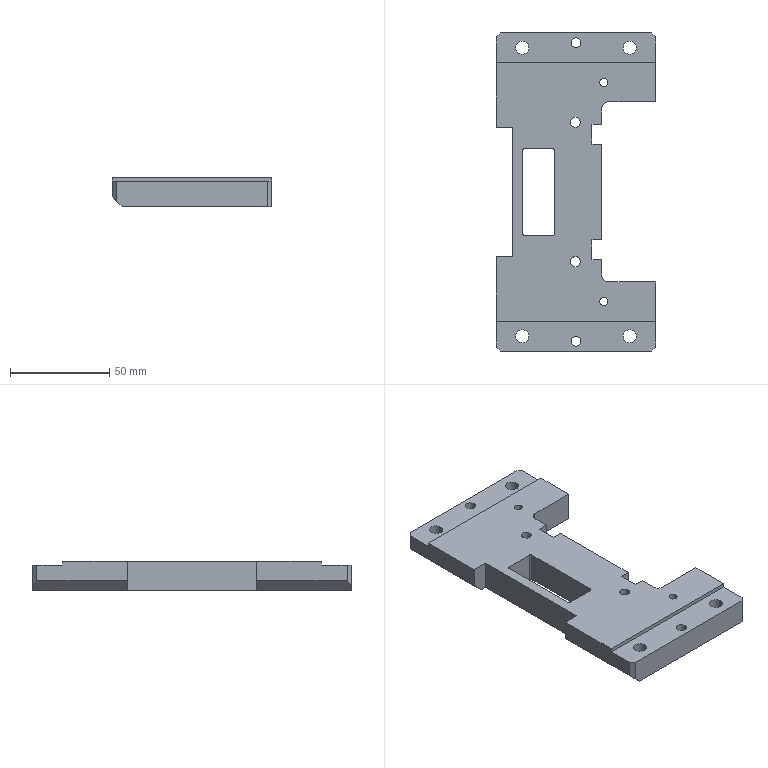Part | NX | features BREP 1 | 1 solid | 134 faces | box 80 x 160 x 15 mm | volume 123294 mm3 | cylinder 64 | plane 40 | cone 30 | commonest cylinder face diameters 3.3 x16 2.5 x8 5 x8 6.6 x8 11 x8 4.2 x6